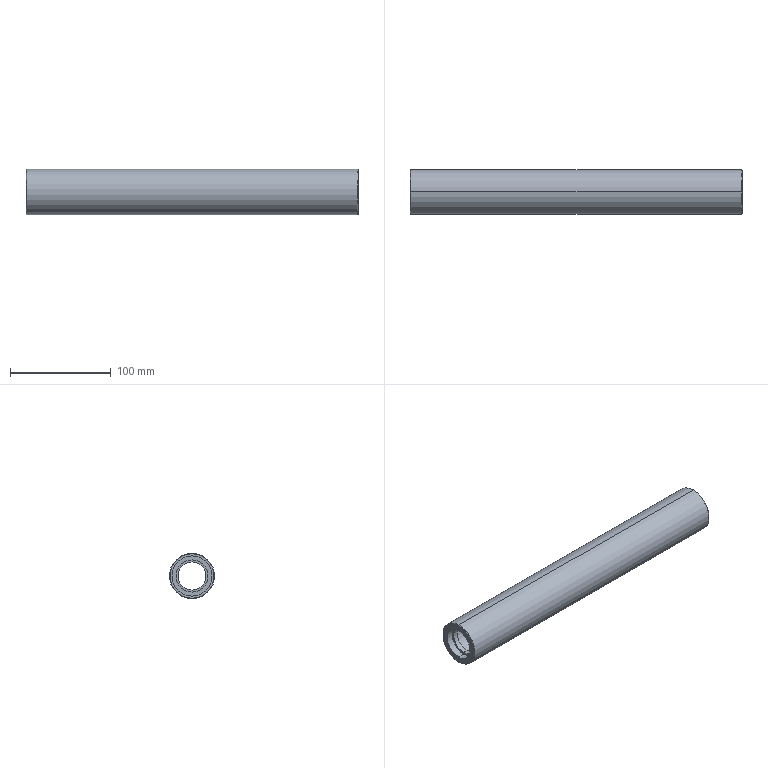Part | SolidWorks | features ICE 4, Chamfer 1, Revolution 1 | 3 solids | 34 faces | box 330 x 45 x 45 mm | volume 212984 mm3 | cylinder 20 | plane 10 | cone 4 | commonest cylinder face diameters 40 x8 28 x4 32 x4 35 x2 45 x2
STEP:
#1=CARTESIAN_POINT('',(23.121,0.,22.));
#2=VERTEX_POINT('',#1);
#3=CARTESIAN_POINT('',(23.121,0.,-22.));
#4=VERTEX_POINT('',#3);
#5=CARTESIAN_POINT('',(23.121,0.,0.));
#6=DIRECTION('',(-1.,0.,0.));
#7=DIRECTION('',(0.,0.,-1.));
#8=AXIS2_PLACEMENT_3D('',#5,#6,#7);
#9=CIRCLE('',#8,22.);
#10=EDGE_CURVE('',#2,#4,#9,.T.);
#11=ORIENTED_EDGE('',*,*,#10,.F.);
#12=CARTESIAN_POINT('',(23.621,0.,22.5));
#13=VERTEX_POINT('',#12);
#14=CARTESIAN_POINT('',(23.121,0.,22.));
#15=DIRECTION('',(0.7071,0.,0.7071));
#16=VECTOR('',#15,1000.);
#17=LINE('',#14,#16);
#18=EDGE_CURVE('',#2,#13,#17,.T.);
#19=ORIENTED_EDGE('',*,*,#18,.T.);
#20=CARTESIAN_POINT('',(23.621,0.,-22.5));
#21=VERTEX_POINT('',#20);
#22=CARTESIAN_POINT('',(23.621,0.,0.));
#23=DIRECTION('',(1.,0.,0.));
#24=DIRECTION('',(0.,0.,-1.));
#25=AXIS2_PLACEMENT_3D('',#22,#23,#24);
#26=CIRCLE('',#25,22.5);
#27=EDGE_CURVE('',#21,#13,#26,.T.);
#28=ORIENTED_EDGE('',*,*,#27,.F.);
#29=CARTESIAN_POINT('',(23.121,0.,-22.));
#30=DIRECTION('',(0.7071,0.,-0.7071));
#31=VECTOR('',#30,1000.);
#32=LINE('',#29,#31);
#33=EDGE_CURVE('',#4,#21,#32,.T.);
#34=ORIENTED_EDGE('',*,*,#33,.F.);
#35=EDGE_LOOP('',(#11,#19,#28,#34));
#36=FACE_OUTER_BOUND('',#35,.T.);
#37=CARTESIAN_POINT('',(23.121,0.,0.));
#38=DIRECTION('',(1.,0.,0.));
#39=DIRECTION('',(0.,0.,-1.));
#40=AXIS2_PLACEMENT_3D('',#37,#38,#39);
#41=CONICAL_SURFACE('',#40,22.,0.7854);
#42=ADVANCED_FACE('',(#36),#41,.T.);
#43=CARTESIAN_POINT('',(353.121,0.,-22.));
#44=VERTEX_POINT('',#43);
#45=CARTESIAN_POINT('',(353.121,0.,22.));
#46=VERTEX_POINT('',#45);
#47=CARTESIAN_POINT('',(353.121,0.,0.));
#48=DIRECTION('',(1.,0.,0.));
#49=DIRECTION('',(0.,0.,1.));
#50=AXIS2_PLACEMENT_3D('',#47,#48,#49);
#51=CIRCLE('',#50,22.);
#52=EDGE_CURVE('',#44,#46,#51,.T.);
#53=ORIENTED_EDGE('',*,*,#52,.F.);
#54=CARTESIAN_POINT('',(352.621,0.,-22.5));
#55=VERTEX_POINT('',#54);
#56=CARTESIAN_POINT('',(352.621,0.,-22.5));
#57=DIRECTION('',(-0.7071,0.,-0.7071));
#58=VECTOR('',#57,1000.);
#59=LINE('',#56,#58);
#60=EDGE_CURVE('',#44,#55,#59,.T.);
#61=ORIENTED_EDGE('',*,*,#60,.T.);
#62=CARTESIAN_POINT('',(352.621,0.,22.5));
#63=VERTEX_POINT('',#62);
#64=CARTESIAN_POINT('',(352.621,0.,0.));
#65=DIRECTION('',(-1.,0.,0.));
#66=DIRECTION('',(0.,0.,1.));
#67=AXIS2_PLACEMENT_3D('',#64,#65,#66);
#68=CIRCLE('',#67,22.5);
#69=EDGE_CURVE('',#63,#55,#68,.T.);
#70=ORIENTED_EDGE('',*,*,#69,.F.);
#71=CARTESIAN_POINT('',(352.621,0.,22.5));
#72=DIRECTION('',(-0.7071,0.,0.7071));
#73=VECTOR('',#72,1000.);
#74=LINE('',#71,#73);
#75=EDGE_CURVE('',#46,#63,#74,.T.);
#76=ORIENTED_EDGE('',*,*,#75,.F.);
#77=EDGE_LOOP('',(#53,#61,#70,#76));
#78=FACE_OUTER_BOUND('',#77,.T.);
#79=CARTESIAN_POINT('',(352.621,0.,0.));
#80=DIRECTION('',(-1.,0.,0.));
#81=DIRECTION('',(0.,0.,1.));
#82=AXIS2_PLACEMENT_3D('',#79,#80,#81);
#83=CONICAL_SURFACE('',#82,22.5,0.7854);
#84=ADVANCED_FACE('',(#78),#83,.T.);
#85=ORIENTED_EDGE('',*,*,#69,.T.);
#86=CARTESIAN_POINT('',(0.,0.,-22.5));
#87=DIRECTION('',(-1.,0.,0.));
#88=VECTOR('',#87,1000.);
#89=LINE('',#86,#88);
#90=EDGE_CURVE('',#55,#21,#89,.T.);
#91=ORIENTED_EDGE('',*,*,#90,.T.);
#92=ORIENTED_EDGE('',*,*,#27,.T.);
#93=CARTESIAN_POINT('',(0.,0.,22.5));
#94=DIRECTION('',(-1.,0.,0.));
#95=VECTOR('',#94,1000.);
#96=LINE('',#93,#95);
#97=EDGE_CURVE('',#63,#13,#96,.T.);
#98=ORIENTED_EDGE('',*,*,#97,.F.);
#99=EDGE_LOOP('',(#85,#91,#92,#98));
#100=FACE_OUTER_BOUND('',#99,.T.);
#101=CARTESIAN_POINT('',(0.,0.,0.));
#102=DIRECTION('',(-1.,0.,0.));
#103=DIRECTION('',(0.,0.,1.));
#104=AXIS2_PLACEMENT_3D('',#101,#102,#103);
#105=CYLINDRICAL_SURFACE('',#104,22.5);
#106=ADVANCED_FACE('',(#100),#105,.T.);
#107=CARTESIAN_POINT('',(35.121,0.,-20.));
#108=VERTEX_POINT('',#107);
#109=CARTESIAN_POINT('',(35.121,0.,20.));
#110=VERTEX_POINT('',#109);
#111=CARTESIAN_POINT('',(35.121,0.,0.));
#112=DIRECTION('',(-1.,0.,0.));
#113=DIRECTION('',(0.,0.,1.));
#114=AXIS2_PLACEMENT_3D('',#111,#112,#113);
#115=CIRCLE('',#114,20.);
#116=EDGE_CURVE('',#108,#110,#115,.T.);
#117=ORIENTED_EDGE('',*,*,#116,.F.);
#118=CARTESIAN_POINT('',(23.121,0.,-20.));
#119=VERTEX_POINT('',#118);
#120=CARTESIAN_POINT('',(0.,0.,-20.));
#121=DIRECTION('',(-1.,0.,0.));
#122=VECTOR('',#121,1000.);
#123=LINE('',#120,#122);
#124=EDGE_CURVE('',#108,#119,#123,.T.);
#125=ORIENTED_EDGE('',*,*,#124,.T.);
#126=CARTESIAN_POINT('',(23.121,0.,20.));
#127=VERTEX_POINT('',#126);
#128=CARTESIAN_POINT('',(23.121,0.,0.));
#129=DIRECTION('',(-1.,0.,0.));
#130=DIRECTION('',(0.,0.,1.));
#131=AXIS2_PLACEMENT_3D('',#128,#129,#130);
#132=CIRCLE('',#131,20.);
#133=EDGE_CURVE('',#119,#127,#132,.T.);
#134=ORIENTED_EDGE('',*,*,#133,.T.);
#135=CARTESIAN_POINT('',(0.,0.,20.));
#136=DIRECTION('',(-1.,0.,0.));
#137=VECTOR('',#136,1000.);
#138=LINE('',#135,#137);
#139=EDGE_CURVE('',#110,#127,#138,.T.);
#140=ORIENTED_EDGE('',*,*,#139,.F.);
#141=EDGE_LOOP('',(#117,#125,#134,#140));
#142=FACE_OUTER_BOUND('',#141,.T.);
#143=CARTESIAN_POINT('',(0.,0.,0.));
#144=DIRECTION('',(-1.,0.,0.));
#145=DIRECTION('',(0.,0.,1.));
#146=AXIS2_PLACEMENT_3D('',#143,#144,#145);
#147=CYLINDRICAL_SURFACE('',#146,20.);
#148=ADVANCED_FACE('',(#142),#147,.F.);
#149=CARTESIAN_POINT('',(341.121,0.,-17.5));
#150=VERTEX_POINT('',#149);
#151=CARTESIAN_POINT('',(341.121,0.,17.5));
#152=VERTEX_POINT('',#151);
#153=CARTESIAN_POINT('',(341.121,0.,0.));
#154=DIRECTION('',(-1.,0.,0.));
#155=DIRECTION('',(0.,0.,1.));
#156=AXIS2_PLACEMENT_3D('',#153,#154,#155);
#157=CIRCLE('',#156,17.5);
#158=EDGE_CURVE('',#150,#152,#157,.T.);
#159=ORIENTED_EDGE('',*,*,#158,.F.);
#160=CARTESIAN_POINT('',(35.121,0.,-17.5));
#161=VERTEX_POINT('',#160);
#162=CARTESIAN_POINT('',(0.,0.,-17.5));
#163=DIRECTION('',(-1.,0.,0.));
#164=VECTOR('',#163,1000.);
#165=LINE('',#162,#164);
#166=EDGE_CURVE('',#150,#161,#165,.T.);
#167=ORIENTED_EDGE('',*,*,#166,.T.);
#168=CARTESIAN_POINT('',(35.121,0.,17.5));
#169=VERTEX_POINT('',#168);
#170=CARTESIAN_POINT('',(35.121,0.,0.));
#171=DIRECTION('',(-1.,0.,0.));
#172=DIRECTION('',(0.,0.,1.));
#173=AXIS2_PLACEMENT_3D('',#170,#171,#172);
#174=CIRCLE('',#173,17.5);
#175=EDGE_CURVE('',#161,#169,#174,.T.);
#176=ORIENTED_EDGE('',*,*,#175,.T.);
#177=CARTESIAN_POINT('',(0.,0.,17.5));
#178=DIRECTION('',(-1.,0.,0.));
#179=VECTOR('',#178,1000.);
#180=LINE('',#177,#179);
#181=EDGE_CURVE('',#152,#169,#180,.T.);
#182=ORIENTED_EDGE('',*,*,#181,.F.);
#183=EDGE_LOOP('',(#159,#167,#176,#182));
#184=FACE_OUTER_BOUND('',#183,.T.);
#185=CARTESIAN_POINT('',(0.,0.,0.));
#186=DIRECTION('',(-1.,0.,0.));
#187=DIRECTION('',(0.,0.,1.));
#188=AXIS2_PLACEMENT_3D('',#185,#186,#187);
#189=CYLINDRICAL_SURFACE('',#188,17.5);
#190=ADVANCED_FACE('',(#184),#189,.F.);
#191=CARTESIAN_POINT('',(353.121,0.,-20.));
#192=VERTEX_POINT('',#191);
#193=CARTESIAN_POINT('',(353.121,0.,20.));
#194=VERTEX_POINT('',#193);
#195=CARTESIAN_POINT('',(353.121,0.,0.));
#196=DIRECTION('',(-1.,0.,0.));
#197=DIRECTION('',(0.,0.,1.));
#198=AXIS2_PLACEMENT_3D('',#195,#196,#197);
#199=CIRCLE('',#198,20.);
#200=EDGE_CURVE('',#192,#194,#199,.T.);
#201=ORIENTED_EDGE('',*,*,#200,.F.);
#202=CARTESIAN_POINT('',(341.121,0.,-20.));
#203=VERTEX_POINT('',#202);
#204=CARTESIAN_POINT('',(0.,0.,-20.));
#205=DIRECTION('',(-1.,0.,0.));
#206=VECTOR('',#205,1000.);
#207=LINE('',#204,#206);
#208=EDGE_CURVE('',#192,#203,#207,.T.);
#209=ORIENTED_EDGE('',*,*,#208,.T.);
#210=CARTESIAN_POINT('',(341.121,0.,20.));
#211=VERTEX_POINT('',#210);
#212=CARTESIAN_POINT('',(341.121,0.,0.));
#213=DIRECTION('',(-1.,0.,0.));
#214=DIRECTION('',(0.,0.,1.));
#215=AXIS2_PLACEMENT_3D('',#212,#213,#214);
#216=CIRCLE('',#215,20.);
#217=EDGE_CURVE('',#203,#211,#216,.T.);
#218=ORIENTED_EDGE('',*,*,#217,.T.);
#219=CARTESIAN_POINT('',(0.,0.,20.));
#220=DIRECTION('',(-1.,0.,0.));
#221=VECTOR('',#220,1000.);
#222=LINE('',#219,#221);
#223=EDGE_CURVE('',#194,#211,#222,.T.);
#224=ORIENTED_EDGE('',*,*,#223,.F.);
#225=EDGE_LOOP('',(#201,#209,#218,#224));
#226=FACE_OUTER_BOUND('',#225,.T.);
#227=CARTESIAN_POINT('',(0.,0.,0.));
#228=DIRECTION('',(-1.,0.,0.));
#229=DIRECTION('',(0.,0.,1.));
#230=AXIS2_PLACEMENT_3D('',#227,#228,#229);
#231=CYLINDRICAL_SURFACE('',#230,20.);
#232=ADVANCED_FACE('',(#226),#231,.F.);
#233=CARTESIAN_POINT('',(353.121,0.,0.));
#234=DIRECTION('',(1.,0.,0.));
#235=DIRECTION('',(0.,0.,1.));
#236=AXIS2_PLACEMENT_3D('',#233,#234,#235);
#237=CIRCLE('',#236,22.);
#238=EDGE_CURVE('',#46,#44,#237,.T.);
#239=ORIENTED_EDGE('',*,*,#238,.T.);
#240=ORIENTED_EDGE('',*,*,#52,.T.);
#241=EDGE_LOOP('',(#239,#240));
#242=FACE_OUTER_BOUND('',#241,.T.);
#243=CARTESIAN_POINT('',(353.121,0.,0.));
#244=DIRECTION('',(-1.,0.,0.));
#245=DIRECTION('',(0.,0.,1.));
#246=AXIS2_PLACEMENT_3D('',#243,#244,#245);
#247=CIRCLE('',#246,20.);
#248=EDGE_CURVE('',#194,#192,#247,.T.);
#249=ORIENTED_EDGE('',*,*,#248,.T.);
#250=ORIENTED_EDGE('',*,*,#200,.T.);
#251=EDGE_LOOP('',(#249,#250));
#252=FACE_BOUND('',#251,.T.);
#253=CARTESIAN_POINT('',(353.121,20.,0.));
#254=DIRECTION('',(-1.,0.,0.));
#255=DIRECTION('',(0.,0.,1.));
#256=AXIS2_PLACEMENT_3D('',#253,#254,#255);
#257=PLANE('',#256);
#258=ADVANCED_FACE('',(#242,#252),#257,.F.);
#259=ORIENTED_EDGE('',*,*,#208,.F.);
#260=ORIENTED_EDGE('',*,*,#248,.F.);
#261=ORIENTED_EDGE('',*,*,#223,.T.);
#262=CARTESIAN_POINT('',(341.121,0.,0.));
#263=DIRECTION('',(-1.,0.,0.));
#264=DIRECTION('',(0.,0.,1.));
#265=AXIS2_PLACEMENT_3D('',#262,#263,#264);
#266=CIRCLE('',#265,20.);
#267=EDGE_CURVE('',#211,#203,#266,.T.);
#268=ORIENTED_EDGE('',*,*,#267,.T.);
#269=EDGE_LOOP('',(#259,#260,#261,#268));
#270=FACE_OUTER_BOUND('',#269,.T.);
#271=CARTESIAN_POINT('',(0.,0.,0.));
#272=DIRECTION('',(-1.,0.,0.));
#273=DIRECTION('',(0.,0.,1.));
#274=AXIS2_PLACEMENT_3D('',#271,#272,#273);
#275=CYLINDRICAL_SURFACE('',#274,20.);
#276=ADVANCED_FACE('',(#270),#275,.F.);
#277=ORIENTED_EDGE('',*,*,#267,.F.);
#278=ORIENTED_EDGE('',*,*,#217,.F.);
#279=EDGE_LOOP('',(#277,#278));
#280=FACE_OUTER_BOUND('',#279,.T.);
#281=CARTESIAN_POINT('',(341.121,0.,0.));
#282=DIRECTION('',(-1.,0.,0.));
#283=DIRECTION('',(0.,0.,1.));
#284=AXIS2_PLACEMENT_3D('',#281,#282,#283);
#285=CIRCLE('',#284,17.5);
#286=EDGE_CURVE('',#152,#150,#285,.T.);
#287=ORIENTED_EDGE('',*,*,#286,.T.);
#288=ORIENTED_EDGE('',*,*,#158,.T.);
#289=EDGE_LOOP('',(#287,#288));
#290=FACE_BOUND('',#289,.T.);
#291=CARTESIAN_POINT('',(341.121,17.5,0.));
#292=DIRECTION('',(-1.,0.,0.));
#293=DIRECTION('',(0.,0.,1.));
#294=AXIS2_PLACEMENT_3D('',#291,#292,#293);
#295=PLANE('',#294);
#296=ADVANCED_FACE('',(#280,#290),#295,.F.);
#297=ORIENTED_EDGE('',*,*,#166,.F.);
#298=ORIENTED_EDGE('',*,*,#286,.F.);
#299=ORIENTED_EDGE('',*,*,#181,.T.);
#300=CARTESIAN_POINT('',(35.121,0.,0.));
#301=DIRECTION('',(-1.,0.,0.));
#302=DIRECTION('',(0.,0.,1.));
#303=AXIS2_PLACEMENT_3D('',#300,#301,#302);
#304=CIRCLE('',#303,17.5);
#305=EDGE_CURVE('',#169,#161,#304,.T.);
#306=ORIENTED_EDGE('',*,*,#305,.T.);
#307=EDGE_LOOP('',(#297,#298,#299,#306));
#308=FACE_OUTER_BOUND('',#307,.T.);
#309=CARTESIAN_POINT('',(0.,0.,0.));
#310=DIRECTION('',(-1.,0.,0.));
#311=DIRECTION('',(0.,0.,1.));
#312=AXIS2_PLACEMENT_3D('',#309,#310,#311);
#313=CYLINDRICAL_SURFACE('',#312,17.5);
#314=ADVANCED_FACE('',(#308),#313,.F.);
#315=ORIENTED_EDGE('',*,*,#305,.F.);
#316=ORIENTED_EDGE('',*,*,#175,.F.);
#317=EDGE_LOOP('',(#315,#316));
#318=FACE_BOUND('',#317,.T.);
#319=CARTESIAN_POINT('',(35.121,0.,0.));
#320=DIRECTION('',(-1.,0.,0.));
#321=DIRECTION('',(0.,0.,1.));
#322=AXIS2_PLACEMENT_3D('',#319,#320,#321);
#323=CIRCLE('',#322,20.);
#324=EDGE_CURVE('',#110,#108,#323,.T.);
#325=ORIENTED_EDGE('',*,*,#324,.T.);
#326=ORIENTED_EDGE('',*,*,#116,.T.);
#327=EDGE_LOOP('',(#325,#326));
#328=FACE_OUTER_BOUND('',#327,.T.);
#329=CARTESIAN_POINT('',(35.121,17.5,0.));
#330=DIRECTION('',(1.,0.,0.));
#331=DIRECTION('',(0.,0.,-1.));
#332=AXIS2_PLACEMENT_3D('',#329,#330,#331);
#333=PLANE('',#332);
#334=ADVANCED_FACE('',(#318,#328),#333,.F.);
#335=ORIENTED_EDGE('',*,*,#124,.F.);
#336=ORIENTED_EDGE('',*,*,#324,.F.);
#337=ORIENTED_EDGE('',*,*,#139,.T.);
#338=CARTESIAN_POINT('',(23.121,0.,0.));
#339=DIRECTION('',(-1.,0.,0.));
#340=DIRECTION('',(0.,0.,1.));
#341=AXIS2_PLACEMENT_3D('',#338,#339,#340);
#342=CIRCLE('',#341,20.);
#343=EDGE_CURVE('',#127,#119,#342,.T.);
#344=ORIENTED_EDGE('',*,*,#343,.T.);
#345=EDGE_LOOP('',(#335,#336,#337,#344));
#346=FACE_OUTER_BOUND('',#345,.T.);
#347=CARTESIAN_POINT('',(0.,0.,0.));
#348=DIRECTION('',(-1.,0.,0.));
#349=DIRECTION('',(0.,0.,1.));
#350=AXIS2_PLACEMENT_3D('',#347,#348,#349);
#351=CYLINDRICAL_SURFACE('',#350,20.);
#352=ADVANCED_FACE('',(#346),#351,.F.);
#353=CARTESIAN_POINT('',(23.121,0.,0.));
#354=DIRECTION('',(-1.,0.,0.));
#355=DIRECTION('',(0.,0.,-1.));
#356=AXIS2_PLACEMENT_3D('',#353,#354,#355);
#357=CIRCLE('',#356,22.);
#358=EDGE_CURVE('',#4,#2,#357,.T.);
#359=ORIENTED_EDGE('',*,*,#358,.T.);
#360=ORIENTED_EDGE('',*,*,#10,.T.);
#361=EDGE_LOOP('',(#359,#360));
#362=FACE_OUTER_BOUND('',#361,.T.);
#363=ORIENTED_EDGE('',*,*,#343,.F.);
#364=ORIENTED_EDGE('',*,*,#133,.F.);
#365=EDGE_LOOP('',(#363,#364));
#366=FACE_BOUND('',#365,.T.);
#367=CARTESIAN_POINT('',(23.121,20.,0.));
#368=DIRECTION('',(1.,0.,0.));
#369=DIRECTION('',(0.,0.,-1.));
#370=AXIS2_PLACEMENT_3D('',#367,#368,#369);
#371=PLANE('',#370);
#372=ADVANCED_FACE('',(#362,#366),#371,.F.);
#373=ORIENTED_EDGE('',*,*,#90,.F.);
#374=CARTESIAN_POINT('',(352.621,0.,0.));
#375=DIRECTION('',(-1.,0.,0.));
#376=DIRECTION('',(0.,0.,1.));
#377=AXIS2_PLACEMENT_3D('',#374,#375,#376);
#378=CIRCLE('',#377,22.5);
#379=EDGE_CURVE('',#55,#63,#378,.T.);
#380=ORIENTED_EDGE('',*,*,#379,.T.);
#381=ORIENTED_EDGE('',*,*,#97,.T.);
#382=CARTESIAN_POINT('',(23.621,0.,0.));
#383=DIRECTION('',(1.,0.,0.));
#384=DIRECTION('',(0.,0.,-1.));
#385=AXIS2_PLACEMENT_3D('',#382,#383,#384);
#386=CIRCLE('',#385,22.5);
#387=EDGE_CURVE('',#13,#21,#386,.T.);
#388=ORIENTED_EDGE('',*,*,#387,.T.);
#389=EDGE_LOOP('',(#373,#380,#381,#388));
#390=FACE_OUTER_BOUND('',#389,.T.);
#391=CARTESIAN_POINT('',(0.,0.,0.));
#392=DIRECTION('',(-1.,0.,0.));
#393=DIRECTION('',(0.,0.,1.));
#394=AXIS2_PLACEMENT_3D('',#391,#392,#393);
#395=CYLINDRICAL_SURFACE('',#394,22.5);
#396=ADVANCED_FACE('',(#390),#395,.T.);
#397=ORIENTED_EDGE('',*,*,#60,.F.);
#398=ORIENTED_EDGE('',*,*,#238,.F.);
#399=ORIENTED_EDGE('',*,*,#75,.T.);
#400=ORIENTED_EDGE('',*,*,#379,.F.);
#401=EDGE_LOOP('',(#397,#398,#399,#400));
#402=FACE_OUTER_BOUND('',#401,.T.);
#403=CARTESIAN_POINT('',(352.621,0.,0.));
#404=DIRECTION('',(-1.,0.,0.));
#405=DIRECTION('',(0.,0.,1.));
#406=AXIS2_PLACEMENT_3D('',#403,#404,#405);
#407=CONICAL_SURFACE('',#406,22.5,0.7854);
#408=ADVANCED_FACE('',(#402),#407,.T.);
#409=ORIENTED_EDGE('',*,*,#18,.F.);
#410=ORIENTED_EDGE('',*,*,#358,.F.);
#411=ORIENTED_EDGE('',*,*,#33,.T.);
#412=ORIENTED_EDGE('',*,*,#387,.F.);
#413=EDGE_LOOP('',(#409,#410,#411,#412));
#414=FACE_OUTER_BOUND('',#413,.T.);
#415=CARTESIAN_POINT('',(23.121,0.,0.));
#416=DIRECTION('',(1.,0.,0.));
#417=DIRECTION('',(0.,0.,-1.));
#418=AXIS2_PLACEMENT_3D('',#415,#416,#417);
#419=CONICAL_SURFACE('',#418,22.,0.7854);
#420=ADVANCED_FACE('',(#414),#419,.T.);
#421=CLOSED_SHELL('',(#42,#84,#106,#148,#190,#232,#258,#276,#296,#314,#334,#352,#372,#396,#408,#420));
#422=MANIFOLD_SOLID_BREP('',#421);
#423=CARTESIAN_POINT('',(346.121,0.,16.));
#424=VERTEX_POINT('',#423);
#425=CARTESIAN_POINT('',(346.121,0.,-16.));
#426=VERTEX_POINT('',#425);
#427=CARTESIAN_POINT('',(346.121,0.,0.));
#428=DIRECTION('',(1.,0.,0.));
#429=DIRECTION('',(0.,0.,-1.));
#430=AXIS2_PLACEMENT_3D('',#427,#428,#429);
#431=CIRCLE('',#430,16.);
#432=EDGE_CURVE('',#424,#426,#431,.T.);
#433=ORIENTED_EDGE('',*,*,#432,.F.);
#434=CARTESIAN_POINT('',(353.121,0.,16.));
#435=VERTEX_POINT('',#434);
#436=CARTESIAN_POINT('',(346.121,0.,16.));
#437=DIRECTION('',(1.,0.,0.));
#438=VECTOR('',#437,1000.);
#439=LINE('',#436,#438);
#440=EDGE_CURVE('',#424,#435,#439,.T.);
#441=ORIENTED_EDGE('',*,*,#440,.T.);
#442=CARTESIAN_POINT('',(353.121,0.,-16.));
#443=VERTEX_POINT('',#442);
#444=CARTESIAN_POINT('',(353.121,0.,0.));
#445=DIRECTION('',(1.,0.,0.));
#446=DIRECTION('',(0.,0.,-1.));
#447=AXIS2_PLACEMENT_3D('',#444,#445,#446);
#448=CIRCLE('',#447,16.);
#449=EDGE_CURVE('',#435,#443,#448,.T.);
#450=ORIENTED_EDGE('',*,*,#449,.T.);
#451=CARTESIAN_POINT('',(346.121,0.,-16.));
#452=DIRECTION('',(1.,0.,0.));
#453=VECTOR('',#452,1000.);
#454=LINE('',#451,#453);
#455=EDGE_CURVE('',#426,#443,#454,.T.);
#456=ORIENTED_EDGE('',*,*,#455,.F.);
#457=EDGE_LOOP('',(#433,#441,#450,#456));
#458=FACE_OUTER_BOUND('',#457,.T.);
#459=CARTESIAN_POINT('',(346.121,0.,0.));
#460=DIRECTION('',(1.,0.,0.));
#461=DIRECTION('',(0.,0.,-1.));
#462=AXIS2_PLACEMENT_3D('',#459,#460,#461);
#463=CYLINDRICAL_SURFACE('',#462,16.);
#464=ADVANCED_FACE('',(#458),#463,.F.);
#465=CARTESIAN_POINT('',(353.121,0.,-20.));
#466=VERTEX_POINT('',#465);
#467=CARTESIAN_POINT('',(353.121,0.,20.));
#468=VERTEX_POINT('',#467);
#469=CARTESIAN_POINT('',(353.121,0.,0.));
#470=DIRECTION('',(1.,0.,0.));
#471=DIRECTION('',(0.,0.,-1.));
#472=AXIS2_PLACEMENT_3D('',#469,#470,#471);
#473=CIRCLE('',#472,20.);
#474=EDGE_CURVE('',#466,#468,#473,.T.);
#475=ORIENTED_EDGE('',*,*,#474,.F.);
#476=CARTESIAN_POINT('',(341.121,0.,-20.));
#477=VERTEX_POINT('',#476);
#478=CARTESIAN_POINT('',(353.121,0.,-20.));
#479=DIRECTION('',(-1.,0.,0.));
#480=VECTOR('',#479,1000.);
#481=LINE('',#478,#480);
#482=EDGE_CURVE('',#466,#477,#481,.T.);
#483=ORIENTED_EDGE('',*,*,#482,.T.);
#484=CARTESIAN_POINT('',(341.121,0.,20.));
#485=VERTEX_POINT('',#484);
#486=CARTESIAN_POINT('',(341.121,0.,0.));
#487=DIRECTION('',(1.,0.,0.));
#488=DIRECTION('',(0.,0.,-1.));
#489=AXIS2_PLACEMENT_3D('',#486,#487,#488);
#490=CIRCLE('',#489,20.);
#491=EDGE_CURVE('',#477,#485,#490,.T.);
#492=ORIENTED_EDGE('',*,*,#491,.T.);
#493=CARTESIAN_POINT('',(353.121,0.,20.));
#494=DIRECTION('',(-1.,0.,0.));
#495=VECTOR('',#494,1000.);
#496=LINE('',#493,#495);
#497=EDGE_CURVE('',#468,#485,#496,.T.);
#498=ORIENTED_EDGE('',*,*,#497,.F.);
#499=EDGE_LOOP('',(#475,#483,#492,#498));
#500=FACE_OUTER_BOUND('',#499,.T.);
#501=CARTESIAN_POINT('',(353.121,0.,0.));
#502=DIRECTION('',(-1.,0.,0.));
#503=DIRECTION('',(0.,0.,1.));
#504=AXIS2_PLACEMENT_3D('',#501,#502,#503);
#505=CYLINDRICAL_SURFACE('',#504,20.);
#506=ADVANCED_FACE('',(#500),#505,.T.);
#507=CARTESIAN_POINT('',(346.121,0.,14.));
#508=VERTEX_POINT('',#507);
#509=CARTESIAN_POINT('',(346.121,0.,-14.));
#510=VERTEX_POINT('',#509);
#511=CARTESIAN_POINT('',(346.121,0.,0.));
#512=DIRECTION('',(1.,0.,0.));
#513=DIRECTION('',(0.,0.,-1.));
#514=AXIS2_PLACEMENT_3D('',#511,#512,#513);
#515=CIRCLE('',#514,14.);
#516=EDGE_CURVE('',#508,#510,#515,.T.);
#517=ORIENTED_EDGE('',*,*,#516,.T.);
#518=CARTESIAN_POINT('',(341.121,0.,-14.));
#519=VERTEX_POINT('',#518);
#520=CARTESIAN_POINT('',(353.121,0.,-14.));
#521=DIRECTION('',(-1.,0.,0.));
#522=VECTOR('',#521,1000.);
#523=LINE('',#520,#522);
#524=EDGE_CURVE('',#510,#519,#523,.T.);
#525=ORIENTED_EDGE('',*,*,#524,.T.);
#526=CARTESIAN_POINT('',(341.121,0.,14.));
#527=VERTEX_POINT('',#526);
#528=CARTESIAN_POINT('',(341.121,0.,0.));
#529=DIRECTION('',(1.,0.,0.));
#530=DIRECTION('',(0.,0.,-1.));
#531=AXIS2_PLACEMENT_3D('',#528,#529,#530);
#532=CIRCLE('',#531,14.);
#533=EDGE_CURVE('',#527,#519,#532,.T.);
#534=ORIENTED_EDGE('',*,*,#533,.F.);
#535=CARTESIAN_POINT('',(353.121,0.,14.));
#536=DIRECTION('',(-1.,0.,0.));
#537=VECTOR('',#536,1000.);
#538=LINE('',#535,#537);
#539=EDGE_CURVE('',#508,#527,#538,.T.);
#540=ORIENTED_EDGE('',*,*,#539,.F.);
#541=EDGE_LOOP('',(#517,#525,#534,#540));
#542=FACE_OUTER_BOUND('',#541,.T.);
#543=CARTESIAN_POINT('',(353.121,0.,0.));
#544=DIRECTION('',(-1.,0.,0.));
#545=DIRECTION('',(0.,0.,1.));
#546=AXIS2_PLACEMENT_3D('',#543,#544,#545);
#547=CYLINDRICAL_SURFACE('',#546,14.);
#548=ADVANCED_FACE('',(#542),#547,.F.);
#549=ORIENTED_EDGE('',*,*,#524,.F.);
#550=CARTESIAN_POINT('',(346.121,0.,0.));
#551=DIRECTION('',(1.,0.,0.));
#552=DIRECTION('',(0.,0.,-1.));
#553=AXIS2_PLACEMENT_3D('',#550,#551,#552);
#554=CIRCLE('',#553,14.);
#555=EDGE_CURVE('',#510,#508,#554,.T.);
#556=ORIENTED_EDGE('',*,*,#555,.T.);
#557=ORIENTED_EDGE('',*,*,#539,.T.);
#558=CARTESIAN_POINT('',(341.121,0.,0.));
#559=DIRECTION('',(1.,0.,0.));
#560=DIRECTION('',(0.,0.,-1.));
#561=AXIS2_PLACEMENT_3D('',#558,#559,#560);
#562=CIRCLE('',#561,14.);
#563=EDGE_CURVE('',#519,#527,#562,.T.);
#564=ORIENTED_EDGE('',*,*,#563,.F.);
#565=EDGE_LOOP('',(#549,#556,#557,#564));
#566=FACE_OUTER_BOUND('',#565,.T.);
#567=CARTESIAN_POINT('',(353.121,0.,0.));
#568=DIRECTION('',(-1.,0.,0.));
#569=DIRECTION('',(0.,0.,1.));
#570=AXIS2_PLACEMENT_3D('',#567,#568,#569);
#571=CYLINDRICAL_SURFACE('',#570,14.);
#572=ADVANCED_FACE('',(#566),#571,.F.);
#573=CARTESIAN_POINT('',(353.121,0.,0.));
#574=DIRECTION('',(1.,0.,0.));
#575=DIRECTION('',(0.,0.,-1.));
#576=AXIS2_PLACEMENT_3D('',#573,#574,#575);
#577=CIRCLE('',#576,16.);
#578=EDGE_CURVE('',#443,#435,#577,.T.);
#579=ORIENTED_EDGE('',*,*,#578,.F.);
#580=ORIENTED_EDGE('',*,*,#449,.F.);
#581=EDGE_LOOP('',(#579,#580));
#582=FACE_BOUND('',#581,.T.);
#583=CARTESIAN_POINT('',(353.121,0.,0.));
#584=DIRECTION('',(1.,0.,0.));
#585=DIRECTION('',(0.,0.,-1.));
#586=AXIS2_PLACEMENT_3D('',#583,#584,#585);
#587=CIRCLE('',#586,20.);
#588=EDGE_CURVE('',#468,#466,#587,.T.);
#589=ORIENTED_EDGE('',*,*,#588,.T.);
#590=ORIENTED_EDGE('',*,*,#474,.T.);
#591=EDGE_LOOP('',(#589,#590));
#592=FACE_OUTER_BOUND('',#591,.T.);
#593=CARTESIAN_POINT('',(353.121,0.,0.));
#594=DIRECTION('',(1.,0.,0.));
#595=DIRECTION('',(0.,0.,-1.));
#596=AXIS2_PLACEMENT_3D('',#593,#594,#595);
#597=PLANE('',#596);
#598=ADVANCED_FACE('',(#582,#592),#597,.T.);
#599=CARTESIAN_POINT('',(341.121,0.,0.));
#600=DIRECTION('',(1.,0.,0.));
#601=DIRECTION('',(0.,0.,-1.));
#602=AXIS2_PLACEMENT_3D('',#599,#600,#601);
#603=CIRCLE('',#602,20.);
#604=EDGE_CURVE('',#485,#477,#603,.T.);
#605=ORIENTED_EDGE('',*,*,#604,.F.);
#606=ORIENTED_EDGE('',*,*,#491,.F.);
#607=EDGE_LOOP('',(#605,#606));
#608=FACE_OUTER_BOUND('',#607,.T.);
#609=ORIENTED_EDGE('',*,*,#533,.T.);
#610=ORIENTED_EDGE('',*,*,#563,.T.);
#611=EDGE_LOOP('',(#609,#610));
#612=FACE_BOUND('',#611,.T.);
#613=CARTESIAN_POINT('',(341.121,0.,0.));
#614=DIRECTION('',(1.,0.,0.));
#615=DIRECTION('',(0.,0.,-1.));
#616=AXIS2_PLACEMENT_3D('',#613,#614,#615);
#617=PLANE('',#616);
#618=ADVANCED_FACE('',(#608,#612),#617,.F.);
#619=ORIENTED_EDGE('',*,*,#482,.F.);
#620=ORIENTED_EDGE('',*,*,#588,.F.);
#621=ORIENTED_EDGE('',*,*,#497,.T.);
#622=ORIENTED_EDGE('',*,*,#604,.T.);
#623=EDGE_LOOP('',(#619,#620,#621,#622));
#624=FACE_OUTER_BOUND('',#623,.T.);
#625=CARTESIAN_POINT('',(353.121,0.,0.));
#626=DIRECTION('',(-1.,0.,0.));
#627=DIRECTION('',(0.,0.,1.));
#628=AXIS2_PLACEMENT_3D('',#625,#626,#627);
#629=CYLINDRICAL_SURFACE('',#628,20.);
#630=ADVANCED_FACE('',(#624),#629,.T.);
#631=ORIENTED_EDGE('',*,*,#440,.F.);
#632=CARTESIAN_POINT('',(346.121,0.,0.));
#633=DIRECTION('',(1.,0.,0.));
#634=DIRECTION('',(0.,0.,-1.));
#635=AXIS2_PLACEMENT_3D('',#632,#633,#634);
#636=CIRCLE('',#635,16.);
#637=EDGE_CURVE('',#426,#424,#636,.T.);
#638=ORIENTED_EDGE('',*,*,#637,.F.);
#639=ORIENTED_EDGE('',*,*,#455,.T.);
#640=ORIENTED_EDGE('',*,*,#578,.T.);
#641=EDGE_LOOP('',(#631,#638,#639,#640));
#642=FACE_OUTER_BOUND('',#641,.T.);
#643=CARTESIAN_POINT('',(346.121,0.,0.));
#644=DIRECTION('',(1.,0.,0.));
#645=DIRECTION('',(0.,0.,-1.));
#646=AXIS2_PLACEMENT_3D('',#643,#644,#645);
#647=CYLINDRICAL_SURFACE('',#646,16.);
#648=ADVANCED_FACE('',(#642),#647,.F.);
#649=ORIENTED_EDGE('',*,*,#516,.F.);
#650=ORIENTED_EDGE('',*,*,#555,.F.);
#651=EDGE_LOOP('',(#649,#650));
#652=FACE_BOUND('',#651,.T.);
#653=ORIENTED_EDGE('',*,*,#637,.T.);
#654=ORIENTED_EDGE('',*,*,#432,.T.);
#655=EDGE_LOOP('',(#653,#654));
#656=FACE_OUTER_BOUND('',#655,.T.);
#657=CARTESIAN_POINT('',(346.121,0.,0.));
#658=DIRECTION('',(1.,0.,0.));
#659=DIRECTION('',(0.,0.,-1.));
#660=AXIS2_PLACEMENT_3D('',#657,#658,#659);
#661=PLANE('',#660);
#662=ADVANCED_FACE('',(#652,#656),#661,.T.);
#663=CLOSED_SHELL('',(#464,#506,#548,#572,#598,#618,#630,#648,#662));
#664=MANIFOLD_SOLID_BREP('',#663);
#665=CARTESIAN_POINT('',(30.121,0.,-16.));
#666=VERTEX_POINT('',#665);
#667=CARTESIAN_POINT('',(30.121,0.,16.));
#668=VERTEX_POINT('',#667);
#669=CARTESIAN_POINT('',(30.121,0.,0.));
#670=DIRECTION('',(-1.,0.,0.));
#671=DIRECTION('',(0.,0.,1.));
#672=AXIS2_PLACEMENT_3D('',#669,#670,#671);
#673=CIRCLE('',#672,16.);
#674=EDGE_CURVE('',#666,#668,#673,.T.);
#675=ORIENTED_EDGE('',*,*,#674,.F.);
#676=CARTESIAN_POINT('',(23.121,0.,-16.));
#677=VERTEX_POINT('',#676);
#678=CARTESIAN_POINT('',(30.121,0.,-16.));
#679=DIRECTION('',(-1.,0.,0.));
#680=VECTOR('',#679,1000.);
#681=LINE('',#678,#680);
#682=EDGE_CURVE('',#666,#677,#681,.T.);
#683=ORIENTED_EDGE('',*,*,#682,.T.);
#684=CARTESIAN_POINT('',(23.121,0.,16.));
#685=VERTEX_POINT('',#684);
#686=CARTESIAN_POINT('',(23.121,0.,0.));
#687=DIRECTION('',(-1.,0.,0.));
#688=DIRECTION('',(0.,0.,1.));
#689=AXIS2_PLACEMENT_3D('',#686,#687,#688);
#690=CIRCLE('',#689,16.);
#691=EDGE_CURVE('',#677,#685,#690,.T.);
#692=ORIENTED_EDGE('',*,*,#691,.T.);
#693=CARTESIAN_POINT('',(30.121,0.,16.));
#694=DIRECTION('',(-1.,0.,0.));
#695=VECTOR('',#694,1000.);
#696=LINE('',#693,#695);
#697=EDGE_CURVE('',#668,#685,#696,.T.);
#698=ORIENTED_EDGE('',*,*,#697,.F.);
#699=EDGE_LOOP('',(#675,#683,#692,#698));
#700=FACE_OUTER_BOUND('',#699,.T.);
#701=CARTESIAN_POINT('',(30.121,0.,0.));
#702=DIRECTION('',(-1.,0.,0.));
#703=DIRECTION('',(0.,0.,1.));
#704=AXIS2_PLACEMENT_3D('',#701,#702,#703);
#705=CYLINDRICAL_SURFACE('',#704,16.);
#706=ADVANCED_FACE('',(#700),#705,.F.);
#707=CARTESIAN_POINT('',(23.121,0.,20.));
#708=VERTEX_POINT('',#707);
#709=CARTESIAN_POINT('',(23.121,0.,-20.));
#710=VERTEX_POINT('',#709);
#711=CARTESIAN_POINT('',(23.121,0.,0.));
#712=DIRECTION('',(-1.,0.,0.));
#713=DIRECTION('',(0.,0.,1.));
#714=AXIS2_PLACEMENT_3D('',#711,#712,#713);
#715=CIRCLE('',#714,20.);
#716=EDGE_CURVE('',#708,#710,#715,.T.);
#717=ORIENTED_EDGE('',*,*,#716,.F.);
#718=CARTESIAN_POINT('',(35.121,0.,20.));
#719=VERTEX_POINT('',#718);
#720=CARTESIAN_POINT('',(23.121,0.,20.));
#721=DIRECTION('',(1.,0.,0.));
#722=VECTOR('',#721,1000.);
#723=LINE('',#720,#722);
#724=EDGE_CURVE('',#708,#719,#723,.T.);
#725=ORIENTED_EDGE('',*,*,#724,.T.);
#726=CARTESIAN_POINT('',(35.121,0.,-20.));
#727=VERTEX_POINT('',#726);
#728=CARTESIAN_POINT('',(35.121,0.,0.));
#729=DIRECTION('',(-1.,0.,0.));
#730=DIRECTION('',(0.,0.,1.));
#731=AXIS2_PLACEMENT_3D('',#728,#729,#730);
#732=CIRCLE('',#731,20.);
#733=EDGE_CURVE('',#719,#727,#732,.T.);
#734=ORIENTED_EDGE('',*,*,#733,.T.);
#735=CARTESIAN_POINT('',(23.121,0.,-20.));
#736=DIRECTION('',(1.,0.,0.));
#737=VECTOR('',#736,1000.);
#738=LINE('',#735,#737);
#739=EDGE_CURVE('',#710,#727,#738,.T.);
#740=ORIENTED_EDGE('',*,*,#739,.F.);
#741=EDGE_LOOP('',(#717,#725,#734,#740));
#742=FACE_OUTER_BOUND('',#741,.T.);
#743=CARTESIAN_POINT('',(23.121,0.,0.));
#744=DIRECTION('',(1.,0.,0.));
#745=DIRECTION('',(0.,0.,-1.));
#746=AXIS2_PLACEMENT_3D('',#743,#744,#745);
#747=CYLINDRICAL_SURFACE('',#746,20.);
#748=ADVANCED_FACE('',(#742),#747,.T.);
#749=CARTESIAN_POINT('',(30.121,0.,-14.));
#750=VERTEX_POINT('',#749);
#751=CARTESIAN_POINT('',(30.121,0.,14.));
#752=VERTEX_POINT('',#751);
#753=CARTESIAN_POINT('',(30.121,0.,0.));
#754=DIRECTION('',(-1.,0.,0.));
#755=DIRECTION('',(0.,0.,1.));
#756=AXIS2_PLACEMENT_3D('',#753,#754,#755);
#757=CIRCLE('',#756,14.);
#758=EDGE_CURVE('',#750,#752,#757,.T.);
#759=ORIENTED_EDGE('',*,*,#758,.T.);
#760=CARTESIAN_POINT('',(35.121,0.,14.));
#761=VERTEX_POINT('',#760);
#762=CARTESIAN_POINT('',(23.121,0.,14.));
#763=DIRECTION('',(1.,0.,0.));
#764=VECTOR('',#763,1000.);
#765=LINE('',#762,#764);
#766=EDGE_CURVE('',#752,#761,#765,.T.);
#767=ORIENTED_EDGE('',*,*,#766,.T.);
#768=CARTESIAN_POINT('',(35.121,0.,-14.));
#769=VERTEX_POINT('',#768);
#770=CARTESIAN_POINT('',(35.121,0.,0.));
#771=DIRECTION('',(-1.,0.,0.));
#772=DIRECTION('',(0.,0.,1.));
#773=AXIS2_PLACEMENT_3D('',#770,#771,#772);
#774=CIRCLE('',#773,14.);
#775=EDGE_CURVE('',#769,#761,#774,.T.);
#776=ORIENTED_EDGE('',*,*,#775,.F.);
#777=CARTESIAN_POINT('',(23.121,0.,-14.));
#778=DIRECTION('',(1.,0.,0.));
#779=VECTOR('',#778,1000.);
#780=LINE('',#777,#779);
#781=EDGE_CURVE('',#750,#769,#780,.T.);
#782=ORIENTED_EDGE('',*,*,#781,.F.);
#783=EDGE_LOOP('',(#759,#767,#776,#782));
#784=FACE_OUTER_BOUND('',#783,.T.);
#785=CARTESIAN_POINT('',(23.121,0.,0.));
#786=DIRECTION('',(1.,0.,0.));
#787=DIRECTION('',(0.,0.,-1.));
#788=AXIS2_PLACEMENT_3D('',#785,#786,#787);
#789=CYLINDRICAL_SURFACE('',#788,14.);
#790=ADVANCED_FACE('',(#784),#789,.F.);
#791=ORIENTED_EDGE('',*,*,#766,.F.);
#792=CARTESIAN_POINT('',(30.121,0.,0.));
#793=DIRECTION('',(-1.,0.,0.));
#794=DIRECTION('',(0.,0.,1.));
#795=AXIS2_PLACEMENT_3D('',#792,#793,#794);
#796=CIRCLE('',#795,14.);
#797=EDGE_CURVE('',#752,#750,#796,.T.);
#798=ORIENTED_EDGE('',*,*,#797,.T.);
#799=ORIENTED_EDGE('',*,*,#781,.T.);
#800=CARTESIAN_POINT('',(35.121,0.,0.));
#801=DIRECTION('',(-1.,0.,0.));
#802=DIRECTION('',(0.,0.,1.));
#803=AXIS2_PLACEMENT_3D('',#800,#801,#802);
#804=CIRCLE('',#803,14.);
#805=EDGE_CURVE('',#761,#769,#804,.T.);
#806=ORIENTED_EDGE('',*,*,#805,.F.);
#807=EDGE_LOOP('',(#791,#798,#799,#806));
#808=FACE_OUTER_BOUND('',#807,.T.);
#809=CARTESIAN_POINT('',(23.121,0.,0.));
#810=DIRECTION('',(1.,0.,0.));
#811=DIRECTION('',(0.,0.,-1.));
#812=AXIS2_PLACEMENT_3D('',#809,#810,#811);
#813=CYLINDRICAL_SURFACE('',#812,14.);
#814=ADVANCED_FACE('',(#808),#813,.F.);
#815=CARTESIAN_POINT('',(23.121,0.,0.));
#816=DIRECTION('',(-1.,0.,0.));
#817=DIRECTION('',(0.,0.,1.));
#818=AXIS2_PLACEMENT_3D('',#815,#816,#817);
#819=CIRCLE('',#818,16.);
#820=EDGE_CURVE('',#685,#677,#819,.T.);
#821=ORIENTED_EDGE('',*,*,#820,.F.);
#822=ORIENTED_EDGE('',*,*,#691,.F.);
#823=EDGE_LOOP('',(#821,#822));
#824=FACE_BOUND('',#823,.T.);
#825=CARTESIAN_POINT('',(23.121,0.,0.));
#826=DIRECTION('',(-1.,0.,0.));
#827=DIRECTION('',(0.,0.,1.));
#828=AXIS2_PLACEMENT_3D('',#825,#826,#827);
#829=CIRCLE('',#828,20.);
#830=EDGE_CURVE('',#710,#708,#829,.T.);
#831=ORIENTED_EDGE('',*,*,#830,.T.);
#832=ORIENTED_EDGE('',*,*,#716,.T.);
#833=EDGE_LOOP('',(#831,#832));
#834=FACE_OUTER_BOUND('',#833,.T.);
#835=CARTESIAN_POINT('',(23.121,0.,0.));
#836=DIRECTION('',(-1.,0.,0.));
#837=DIRECTION('',(0.,0.,1.));
#838=AXIS2_PLACEMENT_3D('',#835,#836,#837);
#839=PLANE('',#838);
#840=ADVANCED_FACE('',(#824,#834),#839,.T.);
#841=CARTESIAN_POINT('',(35.121,0.,0.));
#842=DIRECTION('',(-1.,0.,0.));
#843=DIRECTION('',(0.,0.,1.));
#844=AXIS2_PLACEMENT_3D('',#841,#842,#843);
#845=CIRCLE('',#844,20.);
#846=EDGE_CURVE('',#727,#719,#845,.T.);
#847=ORIENTED_EDGE('',*,*,#846,.F.);
#848=ORIENTED_EDGE('',*,*,#733,.F.);
#849=EDGE_LOOP('',(#847,#848));
#850=FACE_OUTER_BOUND('',#849,.T.);
#851=ORIENTED_EDGE('',*,*,#775,.T.);
#852=ORIENTED_EDGE('',*,*,#805,.T.);
#853=EDGE_LOOP('',(#851,#852));
#854=FACE_BOUND('',#853,.T.);
#855=CARTESIAN_POINT('',(35.121,0.,0.));
#856=DIRECTION('',(-1.,0.,0.));
#857=DIRECTION('',(0.,0.,1.));
#858=AXIS2_PLACEMENT_3D('',#855,#856,#857);
#859=PLANE('',#858);
#860=ADVANCED_FACE('',(#850,#854),#859,.F.);
#861=ORIENTED_EDGE('',*,*,#724,.F.);
#862=ORIENTED_EDGE('',*,*,#830,.F.);
#863=ORIENTED_EDGE('',*,*,#739,.T.);
#864=ORIENTED_EDGE('',*,*,#846,.T.);
#865=EDGE_LOOP('',(#861,#862,#863,#864));
#866=FACE_OUTER_BOUND('',#865,.T.);
#867=CARTESIAN_POINT('',(23.121,0.,0.));
#868=DIRECTION('',(1.,0.,0.));
#869=DIRECTION('',(0.,0.,-1.));
#870=AXIS2_PLACEMENT_3D('',#867,#868,#869);
#871=CYLINDRICAL_SURFACE('',#870,20.);
#872=ADVANCED_FACE('',(#866),#871,.T.);
#873=ORIENTED_EDGE('',*,*,#682,.F.);
#874=CARTESIAN_POINT('',(30.121,0.,0.));
#875=DIRECTION('',(-1.,0.,0.));
#876=DIRECTION('',(0.,0.,1.));
#877=AXIS2_PLACEMENT_3D('',#874,#875,#876);
#878=CIRCLE('',#877,16.);
#879=EDGE_CURVE('',#668,#666,#878,.T.);
#880=ORIENTED_EDGE('',*,*,#879,.F.);
#881=ORIENTED_EDGE('',*,*,#697,.T.);
#882=ORIENTED_EDGE('',*,*,#820,.T.);
#883=EDGE_LOOP('',(#873,#880,#881,#882));
#884=FACE_OUTER_BOUND('',#883,.T.);
#885=CARTESIAN_POINT('',(30.121,0.,0.));
#886=DIRECTION('',(-1.,0.,0.));
#887=DIRECTION('',(0.,0.,1.));
#888=AXIS2_PLACEMENT_3D('',#885,#886,#887);
#889=CYLINDRICAL_SURFACE('',#888,16.);
#890=ADVANCED_FACE('',(#884),#889,.F.);
#891=ORIENTED_EDGE('',*,*,#758,.F.);
#892=ORIENTED_EDGE('',*,*,#797,.F.);
#893=EDGE_LOOP('',(#891,#892));
#894=FACE_BOUND('',#893,.T.);
#895=ORIENTED_EDGE('',*,*,#879,.T.);
#896=ORIENTED_EDGE('',*,*,#674,.T.);
#897=EDGE_LOOP('',(#895,#896));
#898=FACE_OUTER_BOUND('',#897,.T.);
#899=CARTESIAN_POINT('',(30.121,0.,0.));
#900=DIRECTION('',(-1.,0.,0.));
#901=DIRECTION('',(0.,0.,1.));
#902=AXIS2_PLACEMENT_3D('',#899,#900,#901);
#903=PLANE('',#902);
#904=ADVANCED_FACE('',(#894,#898),#903,.T.);
#905=CLOSED_SHELL('',(#706,#748,#790,#814,#840,#860,#872,#890,#904));
#906=MANIFOLD_SOLID_BREP('',#905);
#907=CARTESIAN_POINT('',(0.,0.,0.));
#908=DIRECTION('',(0.,0.,1.));
#909=DIRECTION('',(1.,0.,0.));
#910=AXIS2_PLACEMENT_3D('',#907,#908,#909);
#911=(LENGTH_UNIT()NAMED_UNIT(*)SI_UNIT(.MILLI.,.METRE.));
#912=UNCERTAINTY_MEASURE_WITH_UNIT(LENGTH_MEASURE(0.00001),#911,'','');
#913=(NAMED_UNIT(*)PLANE_ANGLE_UNIT()SI_UNIT($,.RADIAN.));
#914=(NAMED_UNIT(*)SI_UNIT($,.STERADIAN.)SOLID_ANGLE_UNIT());
#915=(GEOMETRIC_REPRESENTATION_CONTEXT(3)GLOBAL_UNCERTAINTY_ASSIGNED_CONTEXT((#912))GLOBAL_UNIT_ASSIGNED_CONTEXT((#911,#913,#914))REPRESENTATION_CONTEXT('',''));
#916=ADVANCED_BREP_SHAPE_REPRESENTATION('',(#422,#664,#906,#910),#915);